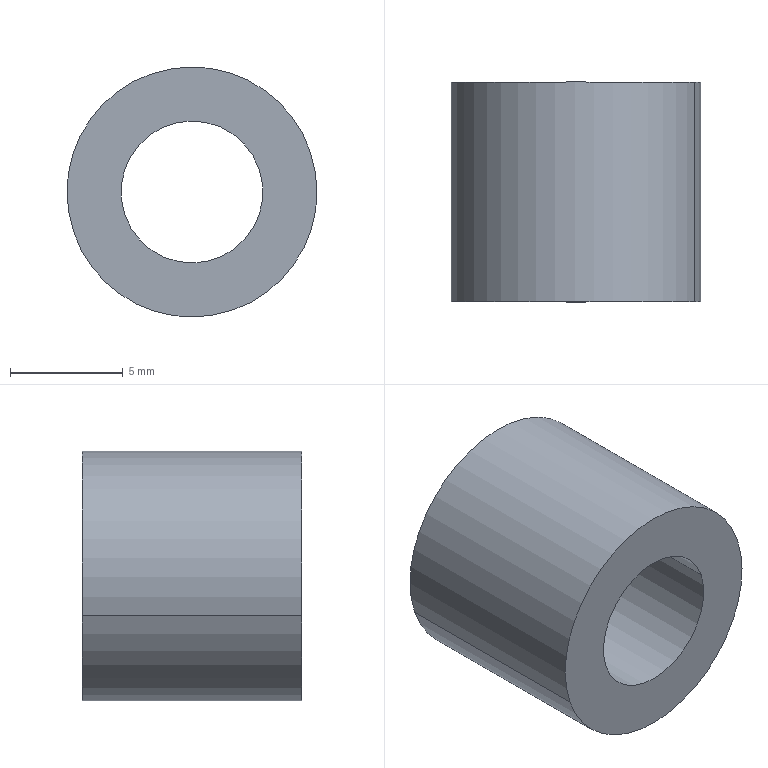Part | STEP file | 2026.6.15-Main Assembly图.sldasm-Part-242 | 1 solid | 6 faces | box 11.1 x 9.75 x 11.1 mm | volume 639.565 mm3 | cylinder 4 | plane 2 | commonest cylinder face diameters 6.3 x2 11.1 x2
STEP:
#1=CARTESIAN_POINT('',(-1516.173,1428.014,3407.079));
#2=VERTEX_POINT('',#1);
#3=CARTESIAN_POINT('',(-1516.173,1437.764,3407.079));
#4=VERTEX_POINT('',#3);
#5=CARTESIAN_POINT('',(-1516.173,1437.764,3407.079));
#6=DIRECTION('',(0.,1.,0.));
#7=VECTOR('',#6,1000.);
#8=LINE('',#5,#7);
#9=EDGE_CURVE('',#2,#4,#8,.T.);
#10=ORIENTED_EDGE('',*,*,#9,.T.);
#11=CARTESIAN_POINT('',(-1510.204,1437.764,3409.094));
#12=VERTEX_POINT('',#11);
#13=CARTESIAN_POINT('',(-1513.188,1437.764,3408.086));
#14=DIRECTION('',(0.,-1.,0.));
#15=DIRECTION('',(0.9474,0.,0.3199));
#16=AXIS2_PLACEMENT_3D('',#13,#14,#15);
#17=CIRCLE('',#16,3.15);
#18=EDGE_CURVE('',#12,#4,#17,.T.);
#19=ORIENTED_EDGE('',*,*,#18,.F.);
#20=CARTESIAN_POINT('',(-1510.204,1428.014,3409.094));
#21=VERTEX_POINT('',#20);
#22=CARTESIAN_POINT('',(-1510.204,1437.764,3409.094));
#23=DIRECTION('',(0.,1.,0.));
#24=VECTOR('',#23,1000.);
#25=LINE('',#22,#24);
#26=EDGE_CURVE('',#21,#12,#25,.T.);
#27=ORIENTED_EDGE('',*,*,#26,.F.);
#28=CARTESIAN_POINT('',(-1513.188,1428.014,3408.086));
#29=DIRECTION('',(0.,-1.,0.));
#30=DIRECTION('',(0.9474,0.,0.3199));
#31=AXIS2_PLACEMENT_3D('',#28,#29,#30);
#32=CIRCLE('',#31,3.15);
#33=EDGE_CURVE('',#21,#2,#32,.T.);
#34=ORIENTED_EDGE('',*,*,#33,.T.);
#35=EDGE_LOOP('',(#10,#19,#27,#34));
#36=FACE_OUTER_BOUND('',#35,.T.);
#37=CARTESIAN_POINT('',(-1513.188,1437.764,3408.086));
#38=DIRECTION('',(0.,-1.,0.));
#39=DIRECTION('',(-0.9474,0.,-0.3199));
#40=AXIS2_PLACEMENT_3D('',#37,#38,#39);
#41=CYLINDRICAL_SURFACE('',#40,3.15);
#42=ADVANCED_FACE('',(#36),#41,.F.);
#43=CARTESIAN_POINT('',(-1507.93,1437.764,3409.862));
#44=VERTEX_POINT('',#43);
#45=CARTESIAN_POINT('',(-1518.447,1437.764,3406.311));
#46=VERTEX_POINT('',#45);
#47=CARTESIAN_POINT('',(-1513.188,1437.764,3408.086));
#48=DIRECTION('',(0.,-1.,0.));
#49=DIRECTION('',(0.9474,0.,0.3199));
#50=AXIS2_PLACEMENT_3D('',#47,#48,#49);
#51=CIRCLE('',#50,5.55);
#52=EDGE_CURVE('',#44,#46,#51,.T.);
#53=ORIENTED_EDGE('',*,*,#52,.F.);
#54=CARTESIAN_POINT('',(-1513.188,1437.764,3408.086));
#55=DIRECTION('',(0.,-1.,0.));
#56=DIRECTION('',(0.9474,0.,0.3199));
#57=AXIS2_PLACEMENT_3D('',#54,#55,#56);
#58=CIRCLE('',#57,5.55);
#59=EDGE_CURVE('',#46,#44,#58,.T.);
#60=ORIENTED_EDGE('',*,*,#59,.F.);
#61=EDGE_LOOP('',(#53,#60));
#62=FACE_OUTER_BOUND('',#61,.T.);
#63=ORIENTED_EDGE('',*,*,#18,.T.);
#64=CARTESIAN_POINT('',(-1513.188,1437.764,3408.086));
#65=DIRECTION('',(0.,-1.,0.));
#66=DIRECTION('',(0.9474,0.,0.3199));
#67=AXIS2_PLACEMENT_3D('',#64,#65,#66);
#68=CIRCLE('',#67,3.15);
#69=EDGE_CURVE('',#4,#12,#68,.T.);
#70=ORIENTED_EDGE('',*,*,#69,.T.);
#71=EDGE_LOOP('',(#63,#70));
#72=FACE_BOUND('',#71,.T.);
#73=CARTESIAN_POINT('',(-1513.188,1437.764,3408.086));
#74=DIRECTION('',(0.,1.,0.));
#75=DIRECTION('',(1.,0.,0.));
#76=AXIS2_PLACEMENT_3D('',#73,#74,#75);
#77=PLANE('',#76);
#78=ADVANCED_FACE('',(#62,#72),#77,.T.);
#79=CARTESIAN_POINT('',(-1507.93,1428.014,3409.862));
#80=VERTEX_POINT('',#79);
#81=CARTESIAN_POINT('',(-1518.447,1428.014,3406.311));
#82=VERTEX_POINT('',#81);
#83=CARTESIAN_POINT('',(-1513.188,1428.014,3408.086));
#84=DIRECTION('',(0.,1.,0.));
#85=DIRECTION('',(0.9474,0.,0.3199));
#86=AXIS2_PLACEMENT_3D('',#83,#84,#85);
#87=CIRCLE('',#86,5.55);
#88=EDGE_CURVE('',#80,#82,#87,.T.);
#89=ORIENTED_EDGE('',*,*,#88,.F.);
#90=CARTESIAN_POINT('',(-1513.188,1428.014,3408.086));
#91=DIRECTION('',(0.,1.,0.));
#92=DIRECTION('',(0.9474,0.,0.3199));
#93=AXIS2_PLACEMENT_3D('',#90,#91,#92);
#94=CIRCLE('',#93,5.55);
#95=EDGE_CURVE('',#82,#80,#94,.T.);
#96=ORIENTED_EDGE('',*,*,#95,.F.);
#97=EDGE_LOOP('',(#89,#96));
#98=FACE_OUTER_BOUND('',#97,.T.);
#99=ORIENTED_EDGE('',*,*,#33,.F.);
#100=CARTESIAN_POINT('',(-1513.188,1428.014,3408.086));
#101=DIRECTION('',(0.,-1.,0.));
#102=DIRECTION('',(0.9474,0.,0.3199));
#103=AXIS2_PLACEMENT_3D('',#100,#101,#102);
#104=CIRCLE('',#103,3.15);
#105=EDGE_CURVE('',#2,#21,#104,.T.);
#106=ORIENTED_EDGE('',*,*,#105,.F.);
#107=EDGE_LOOP('',(#99,#106));
#108=FACE_BOUND('',#107,.T.);
#109=CARTESIAN_POINT('',(-1513.188,1428.014,3408.086));
#110=DIRECTION('',(0.,1.,0.));
#111=DIRECTION('',(1.,0.,0.));
#112=AXIS2_PLACEMENT_3D('',#109,#110,#111);
#113=PLANE('',#112);
#114=ADVANCED_FACE('',(#98,#108),#113,.F.);
#115=CARTESIAN_POINT('',(-1518.447,1437.764,3406.311));
#116=DIRECTION('',(0.,1.,0.));
#117=VECTOR('',#116,1000.);
#118=LINE('',#115,#117);
#119=EDGE_CURVE('',#82,#46,#118,.T.);
#120=ORIENTED_EDGE('',*,*,#119,.T.);
#121=ORIENTED_EDGE('',*,*,#59,.T.);
#122=CARTESIAN_POINT('',(-1507.93,1437.764,3409.862));
#123=DIRECTION('',(0.,1.,0.));
#124=VECTOR('',#123,1000.);
#125=LINE('',#122,#124);
#126=EDGE_CURVE('',#80,#44,#125,.T.);
#127=ORIENTED_EDGE('',*,*,#126,.F.);
#128=ORIENTED_EDGE('',*,*,#88,.T.);
#129=EDGE_LOOP('',(#120,#121,#127,#128));
#130=FACE_OUTER_BOUND('',#129,.T.);
#131=CARTESIAN_POINT('',(-1513.188,1437.764,3408.086));
#132=DIRECTION('',(0.,-1.,0.));
#133=DIRECTION('',(-0.9474,0.,-0.3199));
#134=AXIS2_PLACEMENT_3D('',#131,#132,#133);
#135=CYLINDRICAL_SURFACE('',#134,5.55);
#136=ADVANCED_FACE('',(#130),#135,.T.);
#137=ORIENTED_EDGE('',*,*,#69,.F.);
#138=ORIENTED_EDGE('',*,*,#9,.F.);
#139=ORIENTED_EDGE('',*,*,#105,.T.);
#140=ORIENTED_EDGE('',*,*,#26,.T.);
#141=EDGE_LOOP('',(#137,#138,#139,#140));
#142=FACE_OUTER_BOUND('',#141,.T.);
#143=CARTESIAN_POINT('',(-1513.188,1437.764,3408.086));
#144=DIRECTION('',(0.,-1.,0.));
#145=DIRECTION('',(-0.9474,0.,-0.3199));
#146=AXIS2_PLACEMENT_3D('',#143,#144,#145);
#147=CYLINDRICAL_SURFACE('',#146,3.15);
#148=ADVANCED_FACE('',(#142),#147,.F.);
#149=ORIENTED_EDGE('',*,*,#52,.T.);
#150=ORIENTED_EDGE('',*,*,#119,.F.);
#151=ORIENTED_EDGE('',*,*,#95,.T.);
#152=ORIENTED_EDGE('',*,*,#126,.T.);
#153=EDGE_LOOP('',(#149,#150,#151,#152));
#154=FACE_OUTER_BOUND('',#153,.T.);
#155=CARTESIAN_POINT('',(-1513.188,1437.764,3408.086));
#156=DIRECTION('',(0.,-1.,0.));
#157=DIRECTION('',(-0.9474,0.,-0.3199));
#158=AXIS2_PLACEMENT_3D('',#155,#156,#157);
#159=CYLINDRICAL_SURFACE('',#158,5.55);
#160=ADVANCED_FACE('',(#154),#159,.T.);
#161=CLOSED_SHELL('',(#42,#78,#114,#136,#148,#160));
#162=MANIFOLD_SOLID_BREP('',#161);
#163=CARTESIAN_POINT('',(0.,0.,0.));
#164=DIRECTION('',(0.,0.,1.));
#165=DIRECTION('',(1.,0.,0.));
#166=AXIS2_PLACEMENT_3D('',#163,#164,#165);
#167=(LENGTH_UNIT()NAMED_UNIT(*)SI_UNIT(.MILLI.,.METRE.));
#168=UNCERTAINTY_MEASURE_WITH_UNIT(LENGTH_MEASURE(0.00001),#167,'','');
#169=(NAMED_UNIT(*)PLANE_ANGLE_UNIT()SI_UNIT($,.RADIAN.));
#170=(NAMED_UNIT(*)SI_UNIT($,.STERADIAN.)SOLID_ANGLE_UNIT());
#171=(GEOMETRIC_REPRESENTATION_CONTEXT(3)GLOBAL_UNCERTAINTY_ASSIGNED_CONTEXT((#168))GLOBAL_UNIT_ASSIGNED_CONTEXT((#167,#169,#170))REPRESENTATION_CONTEXT('',''));
#172=ADVANCED_BREP_SHAPE_REPRESENTATION('',(#162,#166),#171);